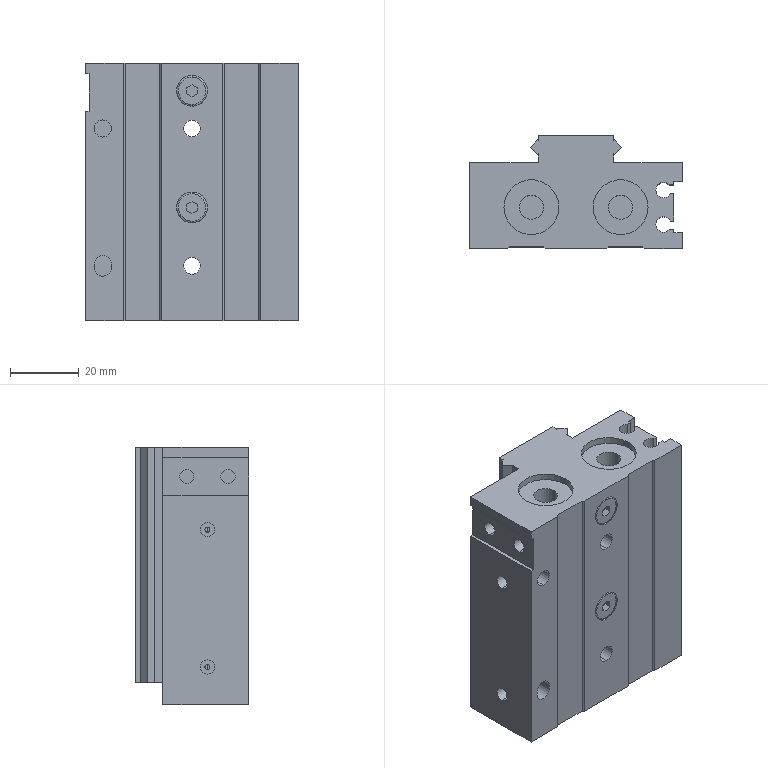Part | SolidWorks | features BaseBody 1 | 1 solid | 145 faces | box 62 x 33 x 75 mm | volume 93823 mm3 | plane 84 | cylinder 57 | spline 4 | commonest cylinder face diameters 4.134 x16 16 x12 5 x5 1.5 x4 4.5 x4 4.917 x4